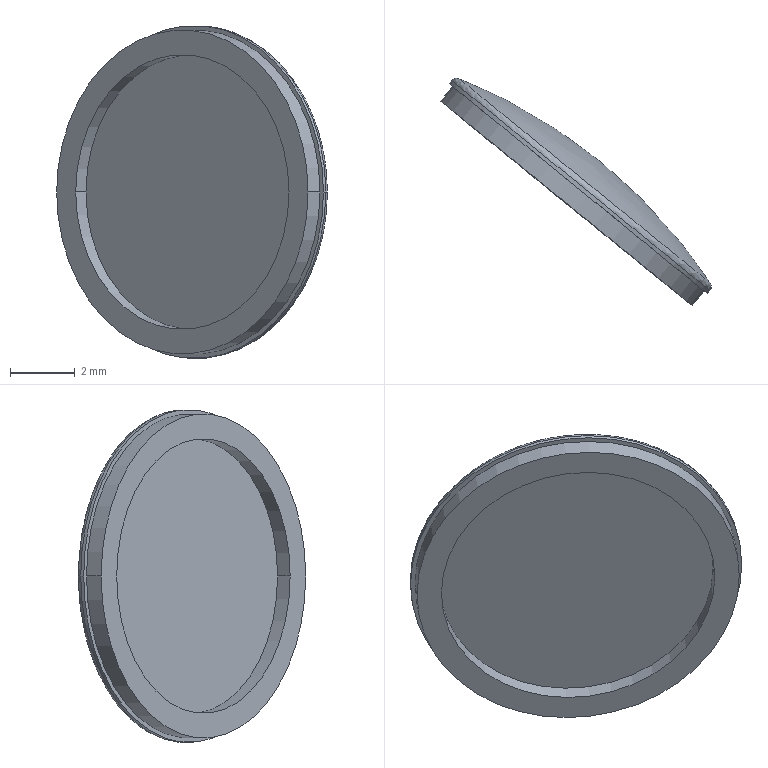Part | SolidWorks | features BaseBody 1 | 1 solid | 12 faces | box 8.353 x 7.015 x 10.277 mm | volume 73.32 mm3 | cylinder 6 | spline 3 | plane 3 | commonest cylinder face diameters 8.485 x2 10 x2 10.277 x2
STEP:
#1=CARTESIAN_POINT('',(566.563,-118.569,298.945));
#2=VERTEX_POINT('',#1);
#3=CARTESIAN_POINT('',(558.59,-112.085,298.945));
#4=VERTEX_POINT('',#3);
#5=CARTESIAN_POINT('',(562.577,-115.327,298.945));
#6=DIRECTION('',(-0.6309,-0.7758,0.000000012));
#7=DIRECTION('',(0.7758,-0.6309,0.));
#8=AXIS2_PLACEMENT_3D('',#5,#6,#7);
#9=CIRCLE('',#8,5.138);
#10=EDGE_CURVE('',#2,#4,#9,.T.);
#11=ORIENTED_EDGE('',*,*,#10,.F.);
#12=CARTESIAN_POINT('',(566.575,-118.332,298.945));
#13=VERTEX_POINT('',#12);
#14=CARTESIAN_POINT('',(566.408,-118.442,298.945));
#15=DIRECTION('',(0.000000024,-0.000000004,1.));
#16=DIRECTION('',(0.7758,-0.6309,-0.000000021));
#17=AXIS2_PLACEMENT_3D('',#14,#15,#16);
#18=CIRCLE('',#17,0.2);
#19=EDGE_CURVE('',#2,#13,#18,.T.);
#20=ORIENTED_EDGE('',*,*,#19,.T.);
#21=CARTESIAN_POINT('',(558.819,-112.025,298.945));
#22=VERTEX_POINT('',#21);
#23=CARTESIAN_POINT('',(562.697,-115.179,298.945));
#24=DIRECTION('',(-0.6309,-0.7758,0.000000012));
#25=DIRECTION('',(-0.7758,0.6309,0.000000021));
#26=AXIS2_PLACEMENT_3D('',#23,#24,#25);
#27=CIRCLE('',#26,4.998);
#28=EDGE_CURVE('',#13,#22,#27,.T.);
#29=ORIENTED_EDGE('',*,*,#28,.T.);
#30=CARTESIAN_POINT('',(558.745,-112.211,298.945));
#31=DIRECTION('',(-0.000000024,0.000000004,-1.));
#32=DIRECTION('',(-0.7758,0.6309,0.000000021));
#33=AXIS2_PLACEMENT_3D('',#30,#31,#32);
#34=CIRCLE('',#33,0.2);
#35=EDGE_CURVE('',#4,#22,#34,.T.);
#36=ORIENTED_EDGE('',*,*,#35,.F.);
#37=EDGE_LOOP('',(#11,#20,#29,#36));
#38=FACE_OUTER_BOUND('',#37,.T.);
#39=CARTESIAN_POINT('',(566.562,-118.568,298.848));
#40=CARTESIAN_POINT('',(566.607,-118.604,301.902));
#41=CARTESIAN_POINT('',(564.947,-117.254,304.083));
#42=CARTESIAN_POINT('',(562.577,-115.327,304.083));
#43=CARTESIAN_POINT('',(560.206,-113.399,304.083));
#44=CARTESIAN_POINT('',(558.546,-112.049,301.902));
#45=CARTESIAN_POINT('',(558.591,-112.085,298.848));
#46=CARTESIAN_POINT('',(566.62,-118.498,298.848));
#47=CARTESIAN_POINT('',(566.664,-118.534,301.902));
#48=CARTESIAN_POINT('',(565.004,-117.184,304.083));
#49=CARTESIAN_POINT('',(562.634,-115.256,304.083));
#50=CARTESIAN_POINT('',(560.263,-113.329,304.083));
#51=CARTESIAN_POINT('',(558.603,-111.979,301.902));
#52=CARTESIAN_POINT('',(558.648,-112.015,298.848));
#53=CARTESIAN_POINT('',(566.624,-118.407,298.849));
#54=CARTESIAN_POINT('',(566.668,-118.443,301.871));
#55=CARTESIAN_POINT('',(565.025,-117.107,304.029));
#56=CARTESIAN_POINT('',(562.68,-115.2,304.029));
#57=CARTESIAN_POINT('',(560.334,-113.292,304.029));
#58=CARTESIAN_POINT('',(558.691,-111.956,301.871));
#59=CARTESIAN_POINT('',(558.736,-111.992,298.849));
#60=CARTESIAN_POINT('',(566.574,-118.332,298.85));
#61=CARTESIAN_POINT('',(566.618,-118.367,301.822));
#62=CARTESIAN_POINT('',(565.003,-117.054,303.943));
#63=CARTESIAN_POINT('',(562.697,-115.179,303.943));
#64=CARTESIAN_POINT('',(560.391,-113.304,303.943));
#65=CARTESIAN_POINT('',(558.776,-111.99,301.822));
#66=CARTESIAN_POINT('',(558.82,-112.026,298.85));
#67=(BOUNDED_SURFACE()B_SPLINE_SURFACE(3,3,((#39,#40,#41,#42,#43,#44,#45),(#46,#47,#48,#49,#50,#51,#52),(#53,#54,#55,#56,#57,#58,#59),(#60,#61,#62,#63,#64,#65,#66)),.UNSPECIFIED.,.F.,.F.,.F.)B_SPLINE_SURFACE_WITH_KNOTS((4,4),(4,3,4),(0.,1.),(0.,0.5,1.),.UNSPECIFIED.)GEOMETRIC_REPRESENTATION_ITEM()RATIONAL_B_SPLINE_SURFACE(((1.,0.8003,0.8003,1.,0.8003,0.8003,1.),(0.8708,0.6969,0.6969,0.8708,0.6969,0.6969,0.8708),(0.8708,0.6969,0.6969,0.8708,0.6969,0.6969,0.8708),(1.,0.8003,0.8003,1.,0.8003,0.8003,1.)))REPRESENTATION_ITEM('')SURFACE());
#68=ADVANCED_FACE('',(#38),#67,.T.);
#69=CARTESIAN_POINT('',(559.158,-112.807,298.945));
#70=VERTEX_POINT('',#69);
#71=CARTESIAN_POINT('',(565.741,-118.16,298.945));
#72=VERTEX_POINT('',#71);
#73=CARTESIAN_POINT('',(562.449,-115.483,298.945));
#74=DIRECTION('',(-0.6309,-0.7758,0.000000012));
#75=DIRECTION('',(0.7758,-0.6309,0.));
#76=AXIS2_PLACEMENT_3D('',#73,#74,#75);
#77=CIRCLE('',#76,4.243);
#78=EDGE_CURVE('',#70,#72,#77,.T.);
#79=ORIENTED_EDGE('',*,*,#78,.F.);
#80=CARTESIAN_POINT('',(558.842,-113.195,298.945));
#81=VERTEX_POINT('',#80);
#82=CARTESIAN_POINT('',(559.,-113.001,298.945));
#83=DIRECTION('',(-0.6309,-0.7758,0.000000012));
#84=VECTOR('',#83,1000.);
#85=LINE('',#82,#84);
#86=EDGE_CURVE('',#70,#81,#85,.T.);
#87=ORIENTED_EDGE('',*,*,#86,.T.);
#88=CARTESIAN_POINT('',(565.425,-118.548,298.945));
#89=VERTEX_POINT('',#88);
#90=CARTESIAN_POINT('',(562.134,-115.871,298.945));
#91=DIRECTION('',(0.6309,0.7758,-0.000000012));
#92=DIRECTION('',(0.7758,-0.6309,0.));
#93=AXIS2_PLACEMENT_3D('',#90,#91,#92);
#94=CIRCLE('',#93,4.243);
#95=EDGE_CURVE('',#89,#81,#94,.T.);
#96=ORIENTED_EDGE('',*,*,#95,.F.);
#97=CARTESIAN_POINT('',(565.583,-118.354,298.945));
#98=DIRECTION('',(-0.6309,-0.7758,0.000000012));
#99=VECTOR('',#98,1000.);
#100=LINE('',#97,#99);
#101=EDGE_CURVE('',#72,#89,#100,.T.);
#102=ORIENTED_EDGE('',*,*,#101,.F.);
#103=EDGE_LOOP('',(#79,#87,#96,#102));
#104=FACE_OUTER_BOUND('',#103,.T.);
#105=CARTESIAN_POINT('',(562.291,-115.677,298.945));
#106=DIRECTION('',(-0.6309,-0.7758,0.000000012));
#107=DIRECTION('',(0.7758,-0.6309,0.));
#108=AXIS2_PLACEMENT_3D('',#105,#106,#107);
#109=CYLINDRICAL_SURFACE('',#108,4.243);
#110=ADVANCED_FACE('',(#104),#109,.F.);
#111=CARTESIAN_POINT('',(566.382,-118.573,298.945));
#112=VERTEX_POINT('',#111);
#113=CARTESIAN_POINT('',(558.623,-112.263,298.945));
#114=VERTEX_POINT('',#113);
#115=CARTESIAN_POINT('',(562.502,-115.418,298.945));
#116=DIRECTION('',(-0.6309,-0.7758,0.000000012));
#117=DIRECTION('',(0.7758,-0.6309,0.));
#118=AXIS2_PLACEMENT_3D('',#115,#116,#117);
#119=CIRCLE('',#118,5.);
#120=EDGE_CURVE('',#112,#114,#119,.T.);
#121=ORIENTED_EDGE('',*,*,#120,.T.);
#122=CARTESIAN_POINT('',(558.254,-112.717,298.945));
#123=VERTEX_POINT('',#122);
#124=CARTESIAN_POINT('',(558.439,-112.49,298.945));
#125=DIRECTION('',(-0.6309,-0.7758,0.000000012));
#126=VECTOR('',#125,1000.);
#127=LINE('',#124,#126);
#128=EDGE_CURVE('',#114,#123,#127,.T.);
#129=ORIENTED_EDGE('',*,*,#128,.T.);
#130=CARTESIAN_POINT('',(566.013,-119.026,298.945));
#131=VERTEX_POINT('',#130);
#132=CARTESIAN_POINT('',(562.134,-115.871,298.945));
#133=DIRECTION('',(-0.6309,-0.7758,0.000000012));
#134=DIRECTION('',(0.7758,-0.6309,0.));
#135=AXIS2_PLACEMENT_3D('',#132,#133,#134);
#136=CIRCLE('',#135,5.);
#137=EDGE_CURVE('',#131,#123,#136,.T.);
#138=ORIENTED_EDGE('',*,*,#137,.F.);
#139=CARTESIAN_POINT('',(566.197,-118.799,298.945));
#140=DIRECTION('',(-0.6309,-0.7758,0.000000012));
#141=VECTOR('',#140,1000.);
#142=LINE('',#139,#141);
#143=EDGE_CURVE('',#112,#131,#142,.T.);
#144=ORIENTED_EDGE('',*,*,#143,.F.);
#145=EDGE_LOOP('',(#121,#129,#138,#144));
#146=FACE_OUTER_BOUND('',#145,.T.);
#147=CARTESIAN_POINT('',(562.318,-115.645,298.945));
#148=DIRECTION('',(-0.6309,-0.7758,0.000000012));
#149=DIRECTION('',(0.7758,-0.6309,0.));
#150=AXIS2_PLACEMENT_3D('',#147,#148,#149);
#151=CYLINDRICAL_SURFACE('',#150,5.);
#152=ADVANCED_FACE('',(#146),#151,.T.);
#153=ORIENTED_EDGE('',*,*,#10,.T.);
#154=CARTESIAN_POINT('',(558.516,-112.176,298.945));
#155=VERTEX_POINT('',#154);
#156=CARTESIAN_POINT('',(558.599,-112.074,298.945));
#157=DIRECTION('',(-0.6309,-0.7758,0.000000012));
#158=VECTOR('',#157,1000.);
#159=LINE('',#156,#158);
#160=EDGE_CURVE('',#4,#155,#159,.T.);
#161=ORIENTED_EDGE('',*,*,#160,.T.);
#162=CARTESIAN_POINT('',(566.489,-118.66,298.945));
#163=VERTEX_POINT('',#162);
#164=CARTESIAN_POINT('',(562.502,-115.418,298.945));
#165=DIRECTION('',(-0.6309,-0.7758,0.000000012));
#166=DIRECTION('',(0.7758,-0.6309,0.));
#167=AXIS2_PLACEMENT_3D('',#164,#165,#166);
#168=CIRCLE('',#167,5.138);
#169=EDGE_CURVE('',#163,#155,#168,.T.);
#170=ORIENTED_EDGE('',*,*,#169,.F.);
#171=CARTESIAN_POINT('',(566.572,-118.558,298.945));
#172=DIRECTION('',(-0.6309,-0.7758,0.000000012));
#173=VECTOR('',#172,1000.);
#174=LINE('',#171,#173);
#175=EDGE_CURVE('',#2,#163,#174,.T.);
#176=ORIENTED_EDGE('',*,*,#175,.F.);
#177=EDGE_LOOP('',(#153,#161,#170,#176));
#178=FACE_OUTER_BOUND('',#177,.T.);
#179=CARTESIAN_POINT('',(562.586,-115.316,298.945));
#180=DIRECTION('',(-0.6309,-0.7758,0.000000012));
#181=DIRECTION('',(0.7758,-0.6309,0.));
#182=AXIS2_PLACEMENT_3D('',#179,#180,#181);
#183=CYLINDRICAL_SURFACE('',#182,5.138);
#184=ADVANCED_FACE('',(#178),#183,.T.);
#185=CARTESIAN_POINT('',(562.449,-115.483,298.945));
#186=DIRECTION('',(-0.6309,-0.7758,0.000000012));
#187=DIRECTION('',(0.7758,-0.6309,0.));
#188=AXIS2_PLACEMENT_3D('',#185,#186,#187);
#189=CIRCLE('',#188,4.243);
#190=EDGE_CURVE('',#72,#70,#189,.T.);
#191=ORIENTED_EDGE('',*,*,#190,.T.);
#192=ORIENTED_EDGE('',*,*,#78,.T.);
#193=EDGE_LOOP('',(#191,#192));
#194=FACE_OUTER_BOUND('',#193,.T.);
#195=CARTESIAN_POINT('',(560.803,-114.145,298.945));
#196=DIRECTION('',(-0.6309,-0.7758,0.000000012));
#197=DIRECTION('',(0.7758,-0.6309,0.));
#198=AXIS2_PLACEMENT_3D('',#195,#196,#197);
#199=PLANE('',#198);
#200=ADVANCED_FACE('',(#194),#199,.T.);
#201=ORIENTED_EDGE('',*,*,#86,.F.);
#202=ORIENTED_EDGE('',*,*,#190,.F.);
#203=ORIENTED_EDGE('',*,*,#101,.T.);
#204=CARTESIAN_POINT('',(562.134,-115.871,298.945));
#205=DIRECTION('',(0.6309,0.7758,-0.000000012));
#206=DIRECTION('',(0.7758,-0.6309,0.));
#207=AXIS2_PLACEMENT_3D('',#204,#205,#206);
#208=CIRCLE('',#207,4.243);
#209=EDGE_CURVE('',#81,#89,#208,.T.);
#210=ORIENTED_EDGE('',*,*,#209,.F.);
#211=EDGE_LOOP('',(#201,#202,#203,#210));
#212=FACE_OUTER_BOUND('',#211,.T.);
#213=CARTESIAN_POINT('',(562.291,-115.677,298.945));
#214=DIRECTION('',(-0.6309,-0.7758,0.000000012));
#215=DIRECTION('',(0.7758,-0.6309,0.));
#216=AXIS2_PLACEMENT_3D('',#213,#214,#215);
#217=CYLINDRICAL_SURFACE('',#216,4.243);
#218=ADVANCED_FACE('',(#212),#217,.F.);
#219=ORIENTED_EDGE('',*,*,#95,.T.);
#220=ORIENTED_EDGE('',*,*,#209,.T.);
#221=EDGE_LOOP('',(#219,#220));
#222=FACE_BOUND('',#221,.T.);
#223=ORIENTED_EDGE('',*,*,#137,.T.);
#224=CARTESIAN_POINT('',(562.134,-115.871,298.945));
#225=DIRECTION('',(-0.6309,-0.7758,0.000000012));
#226=DIRECTION('',(0.7758,-0.6309,0.));
#227=AXIS2_PLACEMENT_3D('',#224,#225,#226);
#228=CIRCLE('',#227,5.);
#229=EDGE_CURVE('',#123,#131,#228,.T.);
#230=ORIENTED_EDGE('',*,*,#229,.T.);
#231=EDGE_LOOP('',(#223,#230));
#232=FACE_OUTER_BOUND('',#231,.T.);
#233=CARTESIAN_POINT('',(558.548,-112.956,298.945));
#234=DIRECTION('',(-0.6309,-0.7758,0.000000012));
#235=DIRECTION('',(0.7758,-0.6309,0.));
#236=AXIS2_PLACEMENT_3D('',#233,#234,#235);
#237=PLANE('',#236);
#238=ADVANCED_FACE('',(#222,#232),#237,.T.);
#239=ORIENTED_EDGE('',*,*,#128,.F.);
#240=CARTESIAN_POINT('',(562.502,-115.418,298.945));
#241=DIRECTION('',(-0.6309,-0.7758,0.000000012));
#242=DIRECTION('',(0.7758,-0.6309,0.));
#243=AXIS2_PLACEMENT_3D('',#240,#241,#242);
#244=CIRCLE('',#243,5.);
#245=EDGE_CURVE('',#114,#112,#244,.T.);
#246=ORIENTED_EDGE('',*,*,#245,.T.);
#247=ORIENTED_EDGE('',*,*,#143,.T.);
#248=ORIENTED_EDGE('',*,*,#229,.F.);
#249=EDGE_LOOP('',(#239,#246,#247,#248));
#250=FACE_OUTER_BOUND('',#249,.T.);
#251=CARTESIAN_POINT('',(562.318,-115.645,298.945));
#252=DIRECTION('',(-0.6309,-0.7758,0.000000012));
#253=DIRECTION('',(0.7758,-0.6309,0.));
#254=AXIS2_PLACEMENT_3D('',#251,#252,#253);
#255=CYLINDRICAL_SURFACE('',#254,5.);
#256=ADVANCED_FACE('',(#250),#255,.T.);
#257=ORIENTED_EDGE('',*,*,#120,.F.);
#258=ORIENTED_EDGE('',*,*,#245,.F.);
#259=EDGE_LOOP('',(#257,#258));
#260=FACE_BOUND('',#259,.T.);
#261=ORIENTED_EDGE('',*,*,#169,.T.);
#262=CARTESIAN_POINT('',(562.502,-115.418,298.945));
#263=DIRECTION('',(-0.6309,-0.7758,0.000000012));
#264=DIRECTION('',(0.7758,-0.6309,0.));
#265=AXIS2_PLACEMENT_3D('',#262,#263,#264);
#266=CIRCLE('',#265,5.138);
#267=EDGE_CURVE('',#155,#163,#266,.T.);
#268=ORIENTED_EDGE('',*,*,#267,.T.);
#269=EDGE_LOOP('',(#261,#268));
#270=FACE_OUTER_BOUND('',#269,.T.);
#271=CARTESIAN_POINT('',(558.57,-112.22,298.945));
#272=DIRECTION('',(-0.6309,-0.7758,0.000000012));
#273=DIRECTION('',(0.7758,-0.6309,0.));
#274=AXIS2_PLACEMENT_3D('',#271,#272,#273);
#275=PLANE('',#274);
#276=ADVANCED_FACE('',(#260,#270),#275,.T.);
#277=ORIENTED_EDGE('',*,*,#160,.F.);
#278=CARTESIAN_POINT('',(562.577,-115.327,298.945));
#279=DIRECTION('',(-0.6309,-0.7758,0.000000012));
#280=DIRECTION('',(0.7758,-0.6309,0.));
#281=AXIS2_PLACEMENT_3D('',#278,#279,#280);
#282=CIRCLE('',#281,5.138);
#283=EDGE_CURVE('',#4,#2,#282,.T.);
#284=ORIENTED_EDGE('',*,*,#283,.T.);
#285=ORIENTED_EDGE('',*,*,#175,.T.);
#286=ORIENTED_EDGE('',*,*,#267,.F.);
#287=EDGE_LOOP('',(#277,#284,#285,#286));
#288=FACE_OUTER_BOUND('',#287,.T.);
#289=CARTESIAN_POINT('',(562.586,-115.316,298.945));
#290=DIRECTION('',(-0.6309,-0.7758,0.000000012));
#291=DIRECTION('',(0.7758,-0.6309,0.));
#292=AXIS2_PLACEMENT_3D('',#289,#290,#291);
#293=CYLINDRICAL_SURFACE('',#292,5.138);
#294=ADVANCED_FACE('',(#288),#293,.T.);
#295=ORIENTED_EDGE('',*,*,#19,.F.);
#296=ORIENTED_EDGE('',*,*,#283,.F.);
#297=ORIENTED_EDGE('',*,*,#35,.T.);
#298=CARTESIAN_POINT('',(562.697,-115.179,298.945));
#299=DIRECTION('',(-0.6309,-0.7758,0.000000012));
#300=DIRECTION('',(-0.7758,0.6309,0.000000021));
#301=AXIS2_PLACEMENT_3D('',#298,#299,#300);
#302=CIRCLE('',#301,4.998);
#303=EDGE_CURVE('',#22,#13,#302,.T.);
#304=ORIENTED_EDGE('',*,*,#303,.T.);
#305=EDGE_LOOP('',(#295,#296,#297,#304));
#306=FACE_OUTER_BOUND('',#305,.T.);
#307=CARTESIAN_POINT('',(558.59,-112.085,298.945));
#308=CARTESIAN_POINT('',(558.59,-112.085,295.912));
#309=CARTESIAN_POINT('',(560.262,-113.444,293.778));
#310=CARTESIAN_POINT('',(562.614,-115.357,293.807));
#311=CARTESIAN_POINT('',(564.967,-117.27,293.835));
#312=CARTESIAN_POINT('',(566.607,-118.604,296.009));
#313=CARTESIAN_POINT('',(566.562,-118.568,299.041));
#314=CARTESIAN_POINT('',(558.647,-112.015,298.945));
#315=CARTESIAN_POINT('',(558.647,-112.015,295.912));
#316=CARTESIAN_POINT('',(560.319,-113.374,293.778));
#317=CARTESIAN_POINT('',(562.671,-115.287,293.807));
#318=CARTESIAN_POINT('',(565.024,-117.2,293.835));
#319=CARTESIAN_POINT('',(566.664,-118.534,296.009));
#320=CARTESIAN_POINT('',(566.62,-118.498,299.041));
#321=CARTESIAN_POINT('',(558.735,-111.992,298.945));
#322=CARTESIAN_POINT('',(558.735,-111.992,295.944));
#323=CARTESIAN_POINT('',(560.389,-113.337,293.832));
#324=CARTESIAN_POINT('',(562.717,-115.23,293.86));
#325=CARTESIAN_POINT('',(565.045,-117.123,293.888));
#326=CARTESIAN_POINT('',(566.668,-118.443,296.04));
#327=CARTESIAN_POINT('',(566.624,-118.407,299.04));
#328=CARTESIAN_POINT('',(558.819,-112.025,298.945));
#329=CARTESIAN_POINT('',(558.819,-112.025,295.995));
#330=CARTESIAN_POINT('',(560.445,-113.347,293.919));
#331=CARTESIAN_POINT('',(562.733,-115.208,293.947));
#332=CARTESIAN_POINT('',(565.022,-117.069,293.974));
#333=CARTESIAN_POINT('',(566.617,-118.367,296.089));
#334=CARTESIAN_POINT('',(566.574,-118.332,299.039));
#335=(BOUNDED_SURFACE()B_SPLINE_SURFACE(3,3,((#307,#308,#309,#310,#311,#312,#313),(#314,#315,#316,#317,#318,#319,#320),(#321,#322,#323,#324,#325,#326,#327),(#328,#329,#330,#331,#332,#333,#334)),.UNSPECIFIED.,.F.,.F.,.F.)B_SPLINE_SURFACE_WITH_KNOTS((4,4),(4,3,4),(0.,1.),(0.,0.5,1.),.UNSPECIFIED.)GEOMETRIC_REPRESENTATION_ITEM()RATIONAL_B_SPLINE_SURFACE(((1.,0.8025,0.8025,1.,0.8025,0.8025,1.),(0.8708,0.6988,0.6988,0.8708,0.6988,0.6988,0.8708),(0.8708,0.6988,0.6988,0.8708,0.6988,0.6988,0.8708),(1.,0.8025,0.8025,1.,0.8025,0.8025,1.)))REPRESENTATION_ITEM('')SURFACE());
#336=ADVANCED_FACE('',(#306),#335,.T.);
#337=ORIENTED_EDGE('',*,*,#303,.F.);
#338=ORIENTED_EDGE('',*,*,#28,.F.);
#339=EDGE_LOOP('',(#337,#338));
#340=FACE_OUTER_BOUND('',#339,.T.);
#341=CARTESIAN_POINT('',(558.283,-112.592,303.796));
#342=CARTESIAN_POINT('',(558.926,-111.801,300.622));
#343=CARTESIAN_POINT('',(558.927,-111.8,297.287));
#344=CARTESIAN_POINT('',(558.287,-112.587,294.111));
#345=CARTESIAN_POINT('',(561.501,-113.908,304.12));
#346=CARTESIAN_POINT('',(562.186,-113.065,300.734));
#347=CARTESIAN_POINT('',(562.188,-113.063,297.177));
#348=CARTESIAN_POINT('',(561.505,-113.903,293.789));
#349=CARTESIAN_POINT('',(564.207,-116.114,304.119));
#350=CARTESIAN_POINT('',(564.893,-115.271,300.733));
#351=CARTESIAN_POINT('',(564.894,-115.269,297.177));
#352=CARTESIAN_POINT('',(564.211,-116.109,293.79));
#353=CARTESIAN_POINT('',(566.147,-118.998,303.794));
#354=CARTESIAN_POINT('',(566.789,-118.209,300.621));
#355=CARTESIAN_POINT('',(566.79,-118.207,297.288));
#356=CARTESIAN_POINT('',(566.151,-118.994,294.114));
#357=(BOUNDED_SURFACE()B_SPLINE_SURFACE(3,3,((#341,#342,#343,#344),(#345,#346,#347,#348),(#349,#350,#351,#352),(#353,#354,#355,#356)),.UNSPECIFIED.,.F.,.F.,.T.)B_SPLINE_SURFACE_WITH_KNOTS((4,4),(4,4),(0.,1.),(0.,1.),.UNSPECIFIED.)GEOMETRIC_REPRESENTATION_ITEM()RATIONAL_B_SPLINE_SURFACE(((1.,0.9682,0.9682,1.),(0.9684,0.9376,0.9376,0.9684),(0.9684,0.9376,0.9376,0.9684),(1.,0.9682,0.9682,1.)))REPRESENTATION_ITEM('')SURFACE());
#358=ADVANCED_FACE('',(#340),#357,.T.);
#359=CLOSED_SHELL('',(#68,#110,#152,#184,#200,#218,#238,#256,#276,#294,#336,#358));
#360=MANIFOLD_SOLID_BREP('',#359);
#361=CARTESIAN_POINT('',(0.,0.,0.));
#362=DIRECTION('',(0.,0.,1.));
#363=DIRECTION('',(1.,0.,0.));
#364=AXIS2_PLACEMENT_3D('',#361,#362,#363);
#365=(LENGTH_UNIT()NAMED_UNIT(*)SI_UNIT(.MILLI.,.METRE.));
#366=UNCERTAINTY_MEASURE_WITH_UNIT(LENGTH_MEASURE(0.00001),#365,'','');
#367=(NAMED_UNIT(*)PLANE_ANGLE_UNIT()SI_UNIT($,.RADIAN.));
#368=(NAMED_UNIT(*)SI_UNIT($,.STERADIAN.)SOLID_ANGLE_UNIT());
#369=(GEOMETRIC_REPRESENTATION_CONTEXT(3)GLOBAL_UNCERTAINTY_ASSIGNED_CONTEXT((#366))GLOBAL_UNIT_ASSIGNED_CONTEXT((#365,#367,#368))REPRESENTATION_CONTEXT('',''));
#370=ADVANCED_BREP_SHAPE_REPRESENTATION('',(#360,#364),#369);